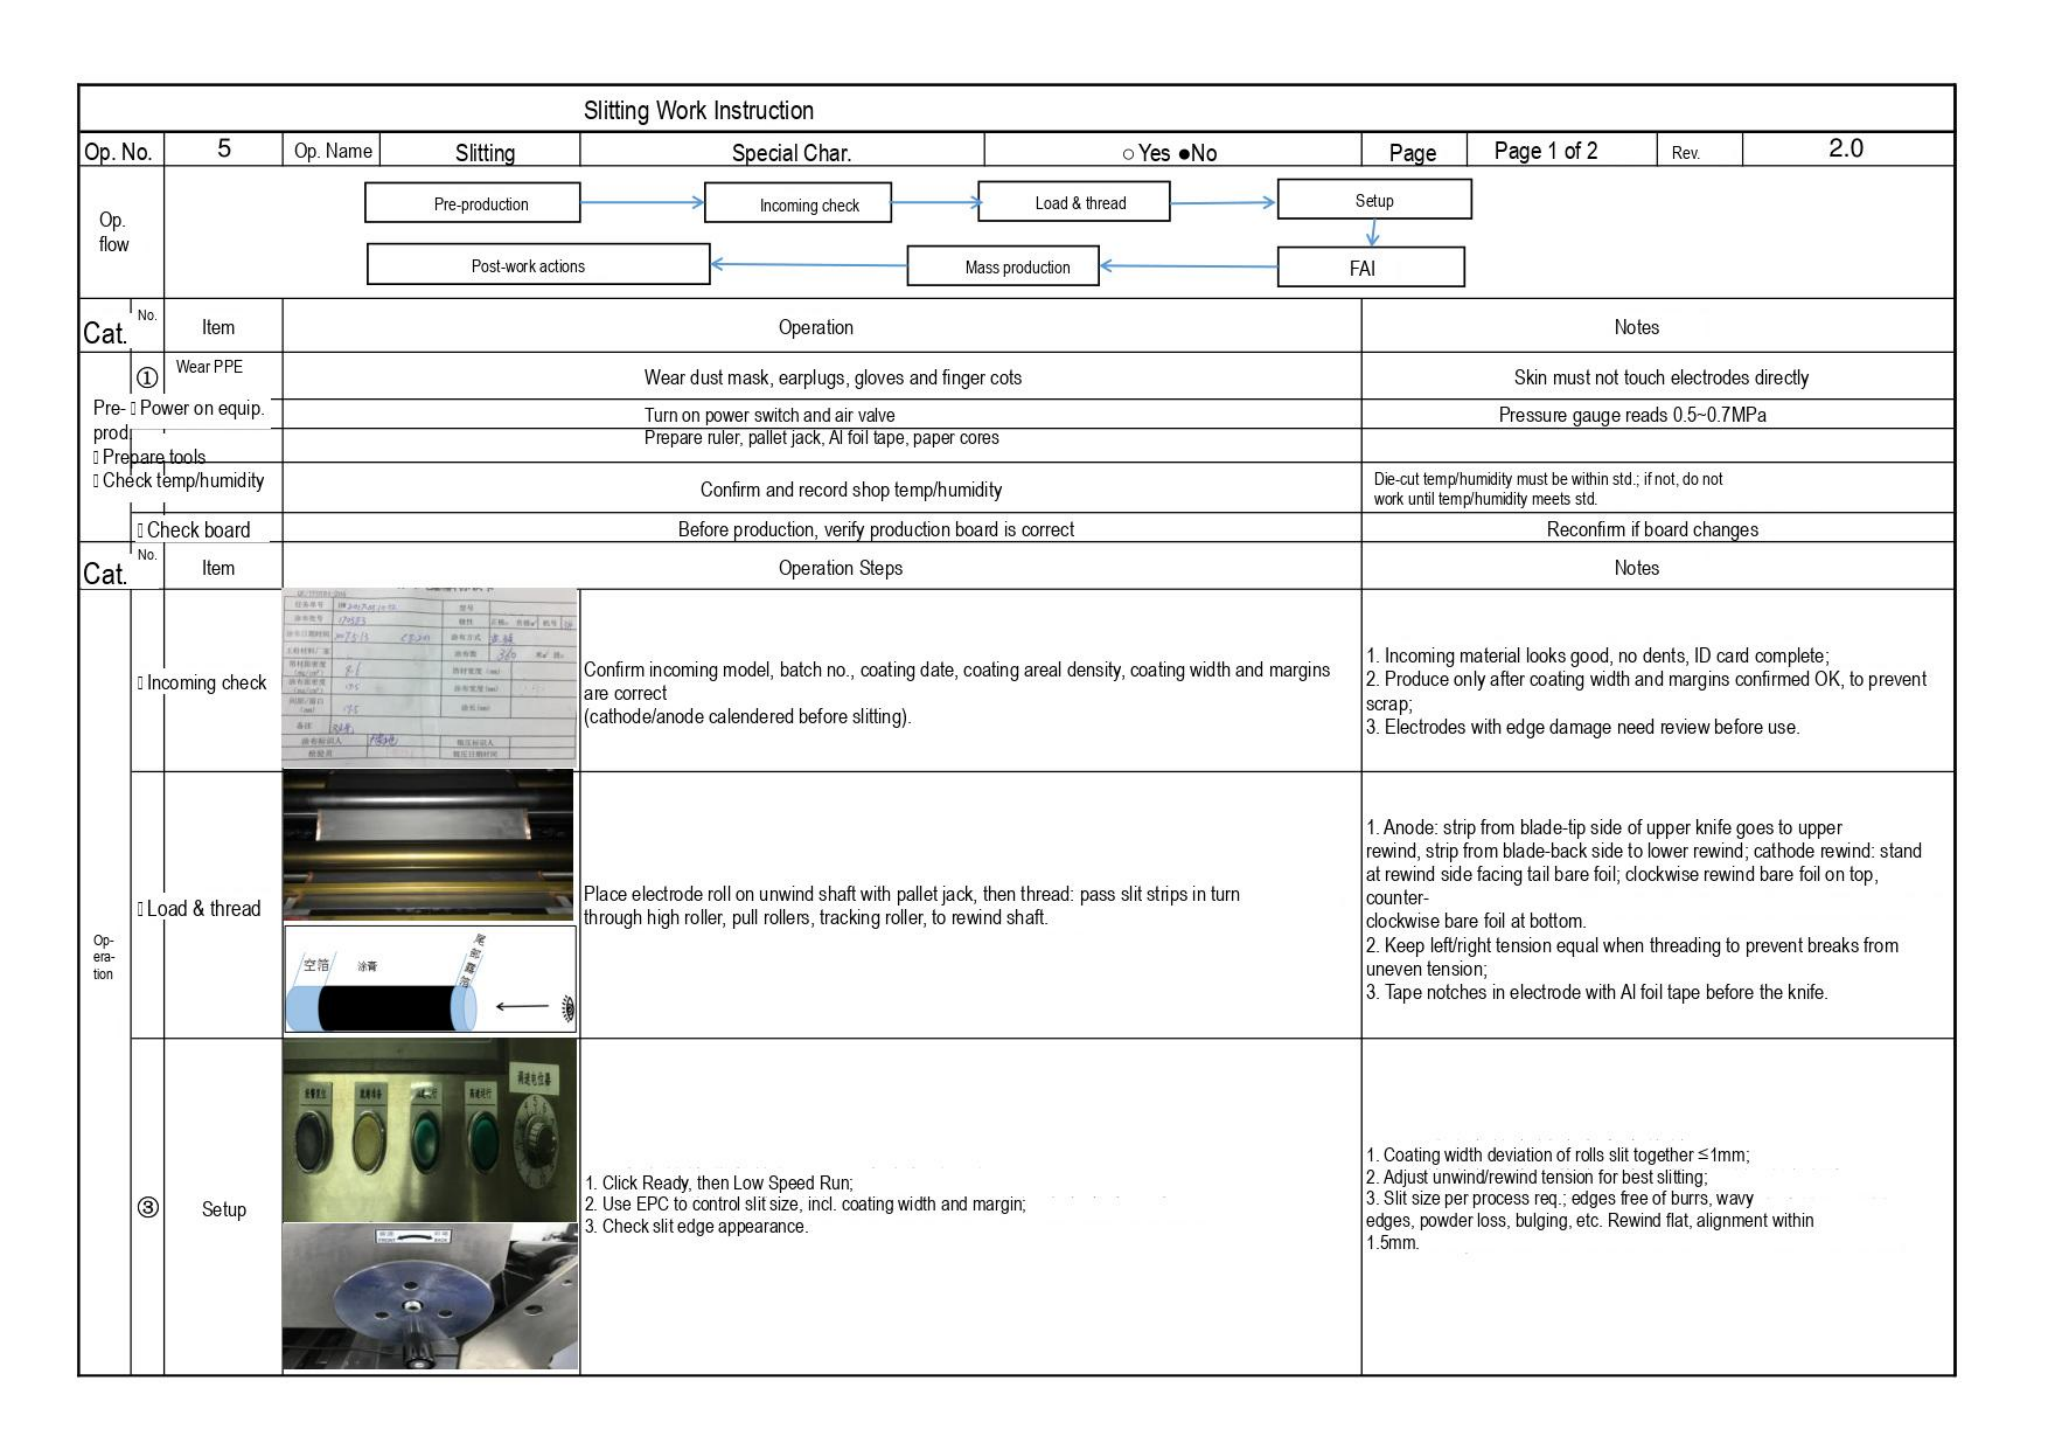# Slitting Work Instruction

| Op. No. | 5 | Op. Name | Slitting | Special Char. | ○Yes ●No | Page | Page 1 of 2 | Rev. | 2.0 |
|---|---|---|---|---|---|---|---|---|---|

**Op. flow**

Pre-production → Incoming check → Load & thread → Setup → FAI → Mass production → Post-work actions

| Cat. | No. | Item | Operation | Notes |
|---|---|---|---|---|
| Pre-prod | ① | Wear PPE | Wear dust mask, earplugs, gloves and finger cots | Skin must not touch electrodes directly |
| | ▯ | Power on equip. | Turn on power switch and air valve | Pressure gauge reads 0.5~0.7MPa |
| | ▯ | Prepare tools | Prepare ruler, pallet jack, Al foil tape, paper cores | |
| | ▯ | Check temp/humidity | Confirm and record shop temp/humidity | Die-cut temp/humidity must be within std.; if not, do not work until temp/humidity meets std. |
| | ▯ | Check board | Before production, verify production board is correct | Reconfirm if board changes |

| Cat. | No. | Item | Operation Steps | Notes |
|---|---|---|---|---|
| Op-era-tion | ▯ | Incoming check | Confirm incoming model, batch no., coating date, coating areal density, coating width and margins are correct<br>(cathode/anode calendered before slitting). | 1. Incoming material looks good, no dents, ID card complete;<br>2. Produce only after coating width and margins confirmed OK, to prevent scrap;<br>3. Electrodes with edge damage need review before use. |
| | ▯ | Load & thread<br>空箔 涂膏 尾部露箔 | Place electrode roll on unwind shaft with pallet jack, then thread: pass slit strips in turn through high roller, pull rollers, tracking roller, to rewind shaft. | 1. Anode: strip from blade-tip side of upper knife goes to upper rewind, strip from blade-back side to lower rewind; cathode rewind: stand at rewind side facing tail bare foil; clockwise rewind bare foil on top, counter-<br>clockwise bare foil at bottom.<br>2. Keep left/right tension equal when threading to prevent breaks from uneven tension;<br>3. Tape notches in electrode with Al foil tape before the knife. |
| | ③ | Setup | 1. Click Ready, then Low Speed Run;<br>2. Use EPC to control slit size, incl. coating width and margin;<br>3. Check slit edge appearance. | 1. Coating width deviation of rolls slit together ≤1mm;<br>2. Adjust unwind/rewind tension for best slitting;<br>3. Slit size per process req.; edges free of burrs, wavy edges, powder loss, bulging, etc. Rewind flat, alignment within 1.5mm. |
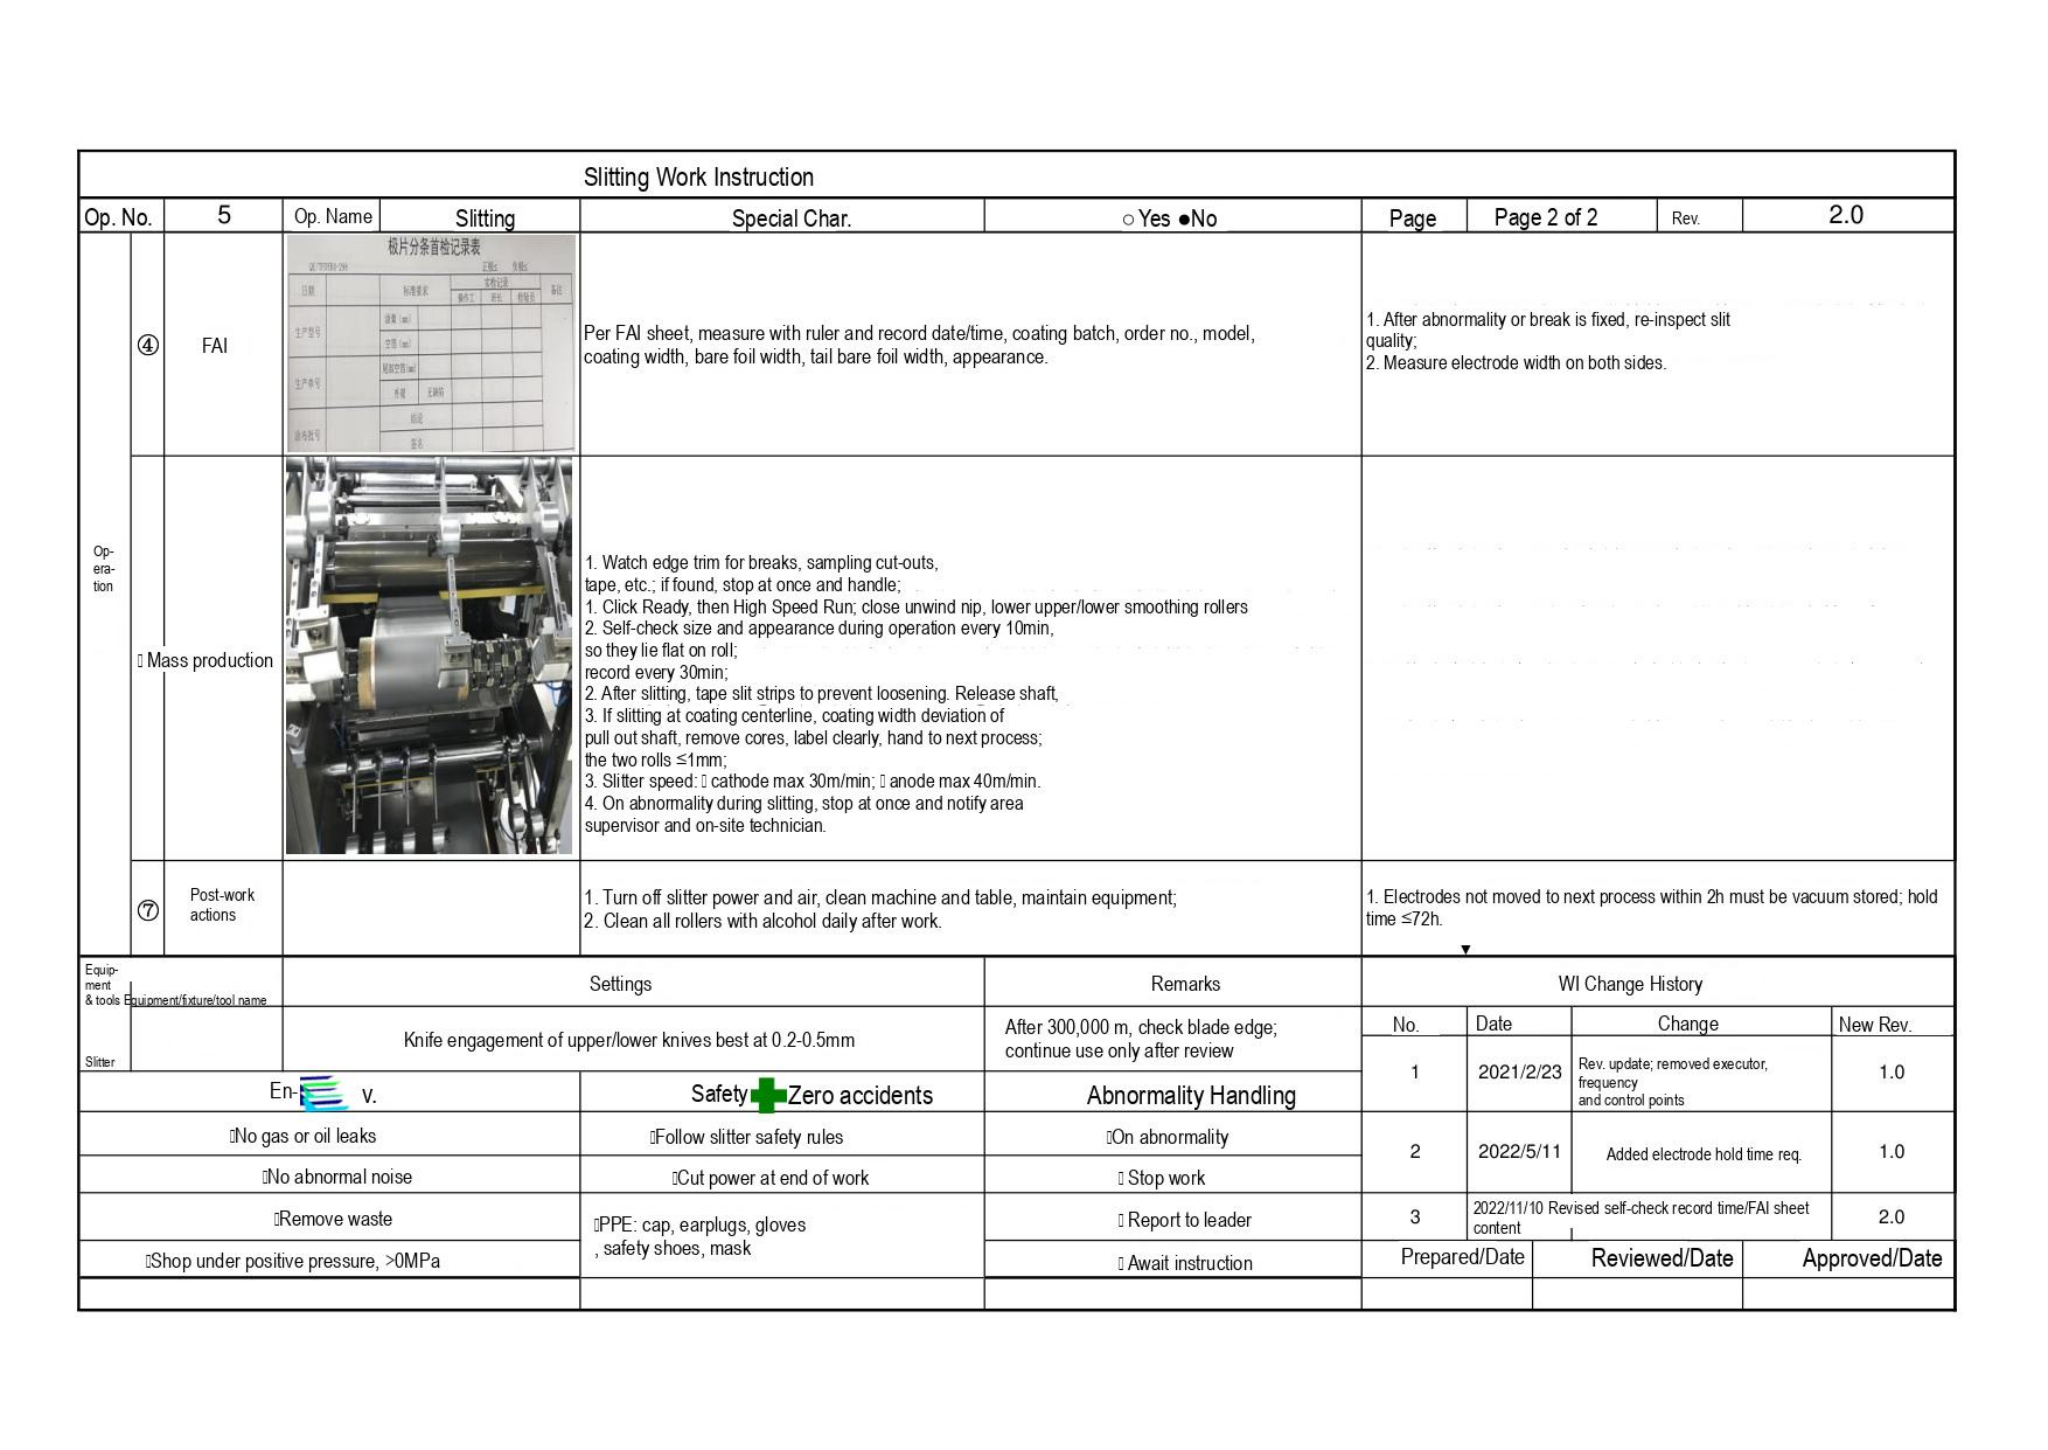Slitting Work Instruction

| Op. No. | 5 | Op. Name | Slitting | Special Char. | ○ Yes ●No | Page | Page 2 of 2 | Rev. | 2.0 |
|---|---|---|---|---|---|---|---|---|---|

| Op-era-tion | | | | | |
|---|---|---|---|---|---|
| | ④ | FAI | 极片分条首检记录表 | Per FAI sheet, measure with ruler and record date/time, coating batch, order no., model, coating width, bare foil width, tail bare foil width, appearance. | 1. After abnormality or break is fixed, re-inspect slit quality;<br>2. Measure electrode width on both sides. |
| | | Mass production | | 1. Watch edge trim for breaks, sampling cut-outs, tape, etc.; if found, stop at once and handle;<br>1. Click Ready, then High Speed Run; close unwind nip, lower upper/lower smoothing rollers<br>2. Self-check size and appearance during operation every 10min, so they lie flat on roll;<br>record every 30min;<br>2. After slitting, tape slit strips to prevent loosening. Release shaft,<br>3. If slitting at coating centerline, coating width deviation of<br>pull out shaft, remove cores, label clearly, hand to next process;<br>the two rolls ≤1mm;<br>3. Slitter speed: cathode max 30m/min; anode max 40m/min.<br>4. On abnormality during slitting, stop at once and notify area supervisor and on-site technician. | |
| | ⑦ | Post-work actions | | 1. Turn off slitter power and air, clean machine and table, maintain equipment;<br>2. Clean all rollers with alcohol daily after work. | 1. Electrodes not moved to next process within 2h must be vacuum stored; hold time ≤72h. |

| Equip-ment & tools | Equipment/fixture/tool name | Settings | Remarks |
|---|---|---|---|
| Slitter | | Knife engagement of upper/lower knives best at 0.2-0.5mm | After 300,000 m, check blade edge; continue use only after review |

| En- v. | Safety Zero accidents | Abnormality Handling |
|---|---|---|
| No gas or oil leaks | Follow slitter safety rules | On abnormality |
| No abnormal noise | Cut power at end of work | Stop work |
| Remove waste | PPE: cap, earplugs, gloves, safety shoes, mask | Report to leader |
| Shop under positive pressure, >0MPa | | Await instruction |

WI Change History

| No. | Date | Change | New Rev. |
|---|---|---|---|
| 1 | 2021/2/23 | Rev. update; removed executor, frequency and control points | 1.0 |
| 2 | 2022/5/11 | Added electrode hold time req. | 1.0 |
| 3 | 2022/11/10 | Revised self-check record time/FAI sheet content | 2.0 |

| Prepared/Date | Reviewed/Date | Approved/Date |
|---|---|---|
| | | |